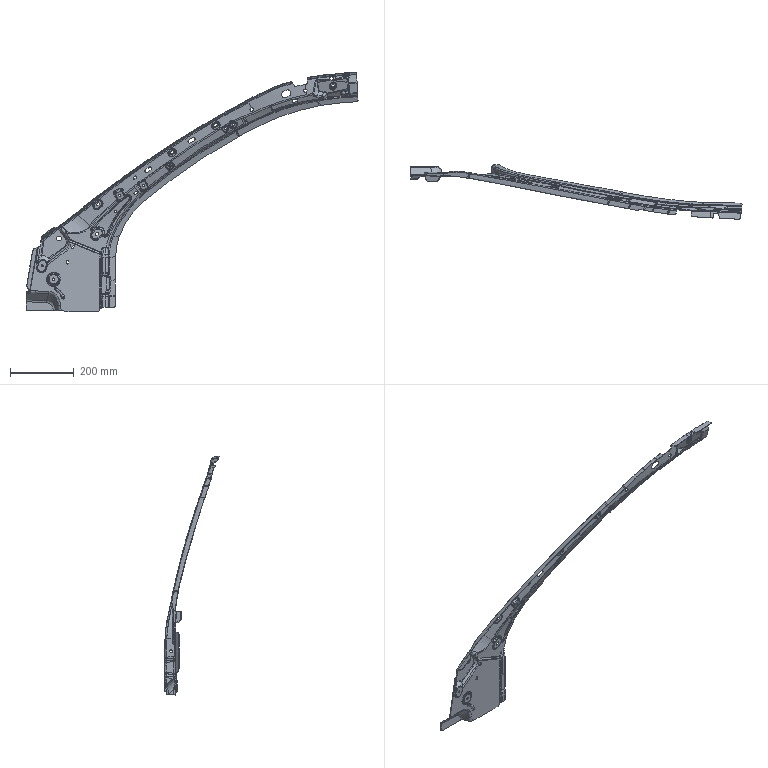Part | STEP file | FNA5401352 | 1 solid | 1517 faces | box 1045 x 172.359 x 753.685 mm | volume 232159 mm3 | spline 1154 | cylinder 231 | plane 93 | sphere 26 | other 9 | torus 4 | commonest cylinder face diameters 6 x27 8.4 x22 7 x16 12 x14 10 x13 3.6 x11